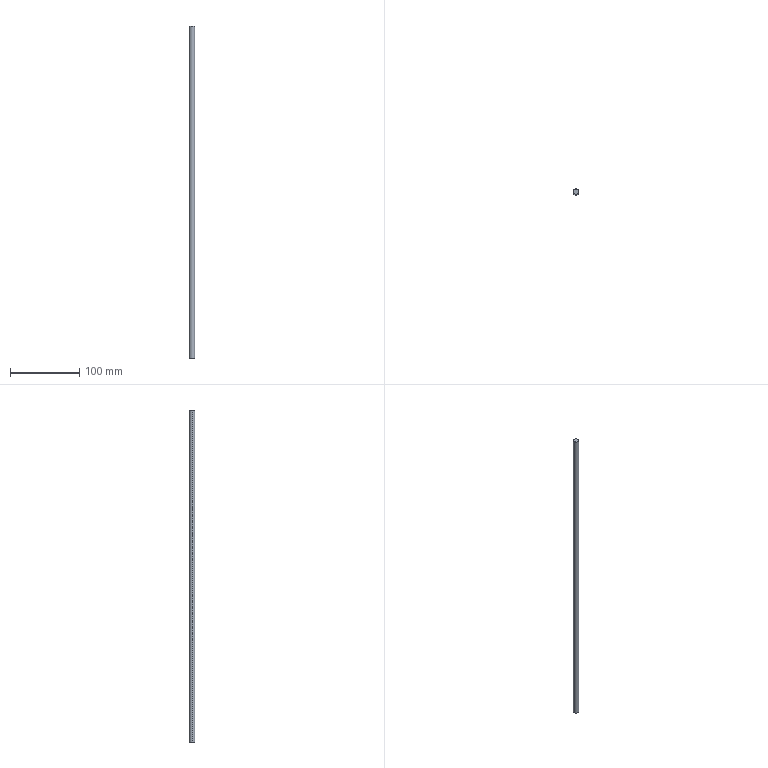Part | STEP file | Sprocket 2 shaft | 1 solid | 4 faces | box 8 x 8 x 480 mm | volume 24127 mm3 | cylinder 2 | plane 2 | commonest cylinder face diameters 8 x2
STEP:
#1=CARTESIAN_POINT('',(0.,0.,0.));
#2=DIRECTION('',(0.,0.,1.));
#3=DIRECTION('',(1.,0.,0.));
#4=AXIS2_PLACEMENT_3D('',#1,#2,#3);
#5=CARTESIAN_POINT('',(4.,0.,480.));
#6=VERTEX_POINT('',#5);
#7=CARTESIAN_POINT('',(-4.,0.,480.));
#8=VERTEX_POINT('',#7);
#9=CARTESIAN_POINT('',(0.,0.,480.));
#10=DIRECTION('',(0.,0.,1.));
#11=DIRECTION('',(1.,0.,0.));
#12=AXIS2_PLACEMENT_3D('',#9,#10,#11);
#13=CIRCLE('',#12,4.);
#14=CARTESIAN_POINT('',(0.,0.,480.));
#15=DIRECTION('',(0.,0.,-1.));
#16=DIRECTION('',(-1.,0.,0.));
#17=AXIS2_PLACEMENT_3D('',#14,#15,#16);
#18=CYLINDRICAL_SURFACE('',#17,4.);
#19=CARTESIAN_POINT('',(3.142,0.));
#20=DIRECTION('',(-1.,0.));
#21=VECTOR('',#20,1.);
#22=LINE('',#19,#21);
#23=(GEOMETRIC_REPRESENTATION_CONTEXT(2)PARAMETRIC_REPRESENTATION_CONTEXT()REPRESENTATION_CONTEXT('',''));
#24=DEFINITIONAL_REPRESENTATION('',(#22),#23);
#25=PCURVE('',#18,#24);
#26=CARTESIAN_POINT('',(0.,0.,480.));
#27=DIRECTION('',(0.,0.,1.));
#28=DIRECTION('',(1.,0.,0.));
#29=AXIS2_PLACEMENT_3D('',#26,#27,#28);
#30=PLANE('',#29);
#31=CARTESIAN_POINT('',(0.,0.));
#32=DIRECTION('',(1.,0.));
#33=AXIS2_PLACEMENT_2D('',#31,#32);
#34=CIRCLE('',#33,4.);
#35=(GEOMETRIC_REPRESENTATION_CONTEXT(2)PARAMETRIC_REPRESENTATION_CONTEXT()REPRESENTATION_CONTEXT('',''));
#36=DEFINITIONAL_REPRESENTATION('',(#34),#35);
#37=PCURVE('',#30,#36);
#38=SURFACE_CURVE('',#13,(#25,#37),.PCURVE_S1.);
#39=EDGE_CURVE('',#6,#8,#38,.T.);
#40=ORIENTED_EDGE('',*,*,#39,.F.);
#41=CARTESIAN_POINT('',(4.,0.,0.));
#42=VERTEX_POINT('',#41);
#43=CARTESIAN_POINT('',(4.,0.,480.));
#44=DIRECTION('',(0.,0.,-1.));
#45=VECTOR('',#44,1.);
#46=LINE('',#43,#45);
#47=CARTESIAN_POINT('',(3.142,0.));
#48=DIRECTION('',(0.,1.));
#49=VECTOR('',#48,1.);
#50=LINE('',#47,#49);
#51=(GEOMETRIC_REPRESENTATION_CONTEXT(2)PARAMETRIC_REPRESENTATION_CONTEXT()REPRESENTATION_CONTEXT('',''));
#52=DEFINITIONAL_REPRESENTATION('',(#50),#51);
#53=PCURVE('',#18,#52);
#54=CARTESIAN_POINT('',(0.,0.,480.));
#55=DIRECTION('',(0.,0.,-1.));
#56=DIRECTION('',(-1.,0.,0.));
#57=AXIS2_PLACEMENT_3D('',#54,#55,#56);
#58=CYLINDRICAL_SURFACE('',#57,4.);
#59=CARTESIAN_POINT('',(3.142,0.));
#60=DIRECTION('',(0.,1.));
#61=VECTOR('',#60,1.);
#62=LINE('',#59,#61);
#63=(GEOMETRIC_REPRESENTATION_CONTEXT(2)PARAMETRIC_REPRESENTATION_CONTEXT()REPRESENTATION_CONTEXT('',''));
#64=DEFINITIONAL_REPRESENTATION('',(#62),#63);
#65=PCURVE('',#58,#64);
#66=SURFACE_CURVE('',#46,(#53,#65),.PCURVE_S1.);
#67=EDGE_CURVE('',#6,#42,#66,.T.);
#68=ORIENTED_EDGE('',*,*,#67,.T.);
#69=CARTESIAN_POINT('',(-4.,0.,0.));
#70=VERTEX_POINT('',#69);
#71=CARTESIAN_POINT('',(0.,0.,0.));
#72=DIRECTION('',(0.,0.,1.));
#73=DIRECTION('',(1.,0.,0.));
#74=AXIS2_PLACEMENT_3D('',#71,#72,#73);
#75=CIRCLE('',#74,4.);
#76=CARTESIAN_POINT('',(3.142,480.));
#77=DIRECTION('',(-1.,0.));
#78=VECTOR('',#77,1.);
#79=LINE('',#76,#78);
#80=(GEOMETRIC_REPRESENTATION_CONTEXT(2)PARAMETRIC_REPRESENTATION_CONTEXT()REPRESENTATION_CONTEXT('',''));
#81=DEFINITIONAL_REPRESENTATION('',(#79),#80);
#82=PCURVE('',#18,#81);
#83=CARTESIAN_POINT('',(0.,0.,0.));
#84=DIRECTION('',(0.,0.,1.));
#85=DIRECTION('',(1.,0.,0.));
#86=AXIS2_PLACEMENT_3D('',#83,#84,#85);
#87=PLANE('',#86);
#88=CARTESIAN_POINT('',(0.,0.));
#89=DIRECTION('',(1.,0.));
#90=AXIS2_PLACEMENT_2D('',#88,#89);
#91=CIRCLE('',#90,4.);
#92=(GEOMETRIC_REPRESENTATION_CONTEXT(2)PARAMETRIC_REPRESENTATION_CONTEXT()REPRESENTATION_CONTEXT('',''));
#93=DEFINITIONAL_REPRESENTATION('',(#91),#92);
#94=PCURVE('',#87,#93);
#95=SURFACE_CURVE('',#75,(#82,#94),.PCURVE_S1.);
#96=EDGE_CURVE('',#42,#70,#95,.T.);
#97=ORIENTED_EDGE('',*,*,#96,.T.);
#98=CARTESIAN_POINT('',(-4.,0.,480.));
#99=DIRECTION('',(0.,0.,-1.));
#100=VECTOR('',#99,1.);
#101=LINE('',#98,#100);
#102=CARTESIAN_POINT('',(0.,0.));
#103=DIRECTION('',(0.,1.));
#104=VECTOR('',#103,1.);
#105=LINE('',#102,#104);
#106=(GEOMETRIC_REPRESENTATION_CONTEXT(2)PARAMETRIC_REPRESENTATION_CONTEXT()REPRESENTATION_CONTEXT('',''));
#107=DEFINITIONAL_REPRESENTATION('',(#105),#106);
#108=PCURVE('',#18,#107);
#109=CARTESIAN_POINT('',(6.283,0.));
#110=DIRECTION('',(0.,1.));
#111=VECTOR('',#110,1.);
#112=LINE('',#109,#111);
#113=(GEOMETRIC_REPRESENTATION_CONTEXT(2)PARAMETRIC_REPRESENTATION_CONTEXT()REPRESENTATION_CONTEXT('',''));
#114=DEFINITIONAL_REPRESENTATION('',(#112),#113);
#115=PCURVE('',#58,#114);
#116=SURFACE_CURVE('',#101,(#108,#115),.PCURVE_S1.);
#117=EDGE_CURVE('',#8,#70,#116,.T.);
#118=ORIENTED_EDGE('',*,*,#117,.F.);
#119=EDGE_LOOP('',(#40,#68,#97,#118));
#120=FACE_BOUND('',#119,.T.);
#121=ADVANCED_FACE('',(#120),#18,.T.);
#122=ORIENTED_EDGE('',*,*,#67,.F.);
#123=CARTESIAN_POINT('',(0.,0.,480.));
#124=DIRECTION('',(0.,0.,1.));
#125=DIRECTION('',(1.,0.,0.));
#126=AXIS2_PLACEMENT_3D('',#123,#124,#125);
#127=CIRCLE('',#126,4.);
#128=CARTESIAN_POINT('',(9.425,0.));
#129=DIRECTION('',(-1.,0.));
#130=VECTOR('',#129,1.);
#131=LINE('',#128,#130);
#132=(GEOMETRIC_REPRESENTATION_CONTEXT(2)PARAMETRIC_REPRESENTATION_CONTEXT()REPRESENTATION_CONTEXT('',''));
#133=DEFINITIONAL_REPRESENTATION('',(#131),#132);
#134=PCURVE('',#58,#133);
#135=CARTESIAN_POINT('',(0.,0.));
#136=DIRECTION('',(1.,0.));
#137=AXIS2_PLACEMENT_2D('',#135,#136);
#138=CIRCLE('',#137,4.);
#139=(GEOMETRIC_REPRESENTATION_CONTEXT(2)PARAMETRIC_REPRESENTATION_CONTEXT()REPRESENTATION_CONTEXT('',''));
#140=DEFINITIONAL_REPRESENTATION('',(#138),#139);
#141=PCURVE('',#30,#140);
#142=SURFACE_CURVE('',#127,(#134,#141),.PCURVE_S1.);
#143=EDGE_CURVE('',#8,#6,#142,.T.);
#144=ORIENTED_EDGE('',*,*,#143,.F.);
#145=ORIENTED_EDGE('',*,*,#117,.T.);
#146=CARTESIAN_POINT('',(0.,0.,0.));
#147=DIRECTION('',(0.,0.,1.));
#148=DIRECTION('',(1.,0.,0.));
#149=AXIS2_PLACEMENT_3D('',#146,#147,#148);
#150=CIRCLE('',#149,4.);
#151=CARTESIAN_POINT('',(9.425,480.));
#152=DIRECTION('',(-1.,0.));
#153=VECTOR('',#152,1.);
#154=LINE('',#151,#153);
#155=(GEOMETRIC_REPRESENTATION_CONTEXT(2)PARAMETRIC_REPRESENTATION_CONTEXT()REPRESENTATION_CONTEXT('',''));
#156=DEFINITIONAL_REPRESENTATION('',(#154),#155);
#157=PCURVE('',#58,#156);
#158=CARTESIAN_POINT('',(0.,0.));
#159=DIRECTION('',(1.,0.));
#160=AXIS2_PLACEMENT_2D('',#158,#159);
#161=CIRCLE('',#160,4.);
#162=(GEOMETRIC_REPRESENTATION_CONTEXT(2)PARAMETRIC_REPRESENTATION_CONTEXT()REPRESENTATION_CONTEXT('',''));
#163=DEFINITIONAL_REPRESENTATION('',(#161),#162);
#164=PCURVE('',#87,#163);
#165=SURFACE_CURVE('',#150,(#157,#164),.PCURVE_S1.);
#166=EDGE_CURVE('',#70,#42,#165,.T.);
#167=ORIENTED_EDGE('',*,*,#166,.T.);
#168=EDGE_LOOP('',(#122,#144,#145,#167));
#169=FACE_BOUND('',#168,.T.);
#170=ADVANCED_FACE('',(#169),#58,.T.);
#171=ORIENTED_EDGE('',*,*,#143,.T.);
#172=ORIENTED_EDGE('',*,*,#39,.T.);
#173=EDGE_LOOP('',(#171,#172));
#174=FACE_BOUND('',#173,.T.);
#175=ADVANCED_FACE('',(#174),#30,.T.);
#176=ORIENTED_EDGE('',*,*,#166,.F.);
#177=ORIENTED_EDGE('',*,*,#96,.F.);
#178=EDGE_LOOP('',(#176,#177));
#179=FACE_BOUND('',#178,.T.);
#180=ADVANCED_FACE('',(#179),#87,.F.);
#181=CLOSED_SHELL('',(#121,#170,#175,#180));
#182=MANIFOLD_SOLID_BREP('',#181);
#183=(LENGTH_UNIT()NAMED_UNIT(*)SI_UNIT(.MILLI.,.METRE.));
#184=UNCERTAINTY_MEASURE_WITH_UNIT(LENGTH_MEASURE(0.0000001),#183,'','');
#185=(NAMED_UNIT(*)PLANE_ANGLE_UNIT()SI_UNIT($,.RADIAN.));
#186=(NAMED_UNIT(*)SI_UNIT($,.STERADIAN.)SOLID_ANGLE_UNIT());
#187=(GEOMETRIC_REPRESENTATION_CONTEXT(3)GLOBAL_UNCERTAINTY_ASSIGNED_CONTEXT((#184))GLOBAL_UNIT_ASSIGNED_CONTEXT((#183,#185,#186))REPRESENTATION_CONTEXT('',''));
#188=ADVANCED_BREP_SHAPE_REPRESENTATION('',(#4,#182),#187);